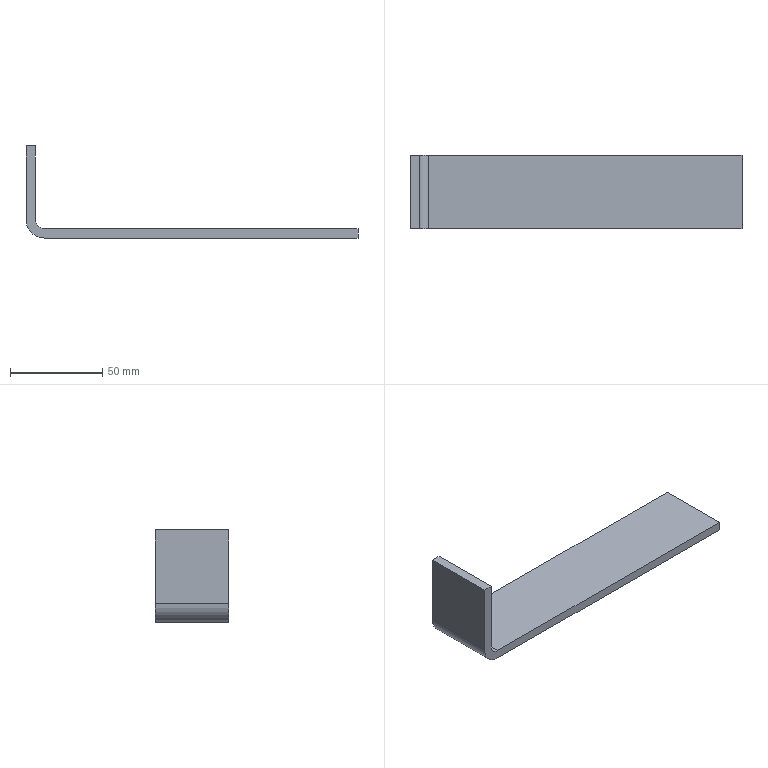Part | SolidWorks | features BaseBody 1 | 1 solid | 10 faces | box 180 x 40 x 50 mm | volume 44356 mm3 | plane 8 | cylinder 2 | commonest cylinder face diameters 10 x1 20 x1
STEP:
#1=CARTESIAN_POINT('',(0.,40.,0.));
#2=VERTEX_POINT('',#1);
#3=CARTESIAN_POINT('',(-170.,40.,0.));
#4=VERTEX_POINT('',#3);
#5=CARTESIAN_POINT('',(-90.,40.,0.));
#6=DIRECTION('',(-1.,0.,0.));
#7=VECTOR('',#6,1000.);
#8=LINE('',#5,#7);
#9=EDGE_CURVE('',#2,#4,#8,.T.);
#10=ORIENTED_EDGE('',*,*,#9,.F.);
#11=CARTESIAN_POINT('',(0.,0.,0.));
#12=VERTEX_POINT('',#11);
#13=CARTESIAN_POINT('',(0.,20.,0.));
#14=DIRECTION('',(0.,1.,0.));
#15=VECTOR('',#14,1000.);
#16=LINE('',#13,#15);
#17=EDGE_CURVE('',#12,#2,#16,.T.);
#18=ORIENTED_EDGE('',*,*,#17,.F.);
#19=CARTESIAN_POINT('',(-170.,0.,0.));
#20=VERTEX_POINT('',#19);
#21=CARTESIAN_POINT('',(-90.,0.,0.));
#22=DIRECTION('',(1.,0.,0.));
#23=VECTOR('',#22,1000.);
#24=LINE('',#21,#23);
#25=EDGE_CURVE('',#20,#12,#24,.T.);
#26=ORIENTED_EDGE('',*,*,#25,.F.);
#27=CARTESIAN_POINT('',(-170.,20.,0.));
#28=DIRECTION('',(0.,-1.,0.));
#29=VECTOR('',#28,1000.);
#30=LINE('',#27,#29);
#31=EDGE_CURVE('',#4,#20,#30,.T.);
#32=ORIENTED_EDGE('',*,*,#31,.F.);
#33=EDGE_LOOP('',(#10,#18,#26,#32));
#34=FACE_OUTER_BOUND('',#33,.T.);
#35=CARTESIAN_POINT('',(-90.,20.,0.));
#36=DIRECTION('',(0.,0.,1.));
#37=DIRECTION('',(1.,0.,0.));
#38=AXIS2_PLACEMENT_3D('',#35,#36,#37);
#39=PLANE('',#38);
#40=ADVANCED_FACE('',(#34),#39,.F.);
#41=ORIENTED_EDGE('',*,*,#31,.T.);
#42=CARTESIAN_POINT('',(-180.,0.,10.));
#43=VERTEX_POINT('',#42);
#44=CARTESIAN_POINT('',(-170.,0.,10.));
#45=DIRECTION('',(0.,1.,0.));
#46=DIRECTION('',(0.,0.,1.));
#47=AXIS2_PLACEMENT_3D('',#44,#45,#46);
#48=CIRCLE('',#47,10.);
#49=EDGE_CURVE('',#20,#43,#48,.T.);
#50=ORIENTED_EDGE('',*,*,#49,.T.);
#51=CARTESIAN_POINT('',(-180.,40.,10.));
#52=VERTEX_POINT('',#51);
#53=CARTESIAN_POINT('',(-180.,20.,10.));
#54=DIRECTION('',(0.,1.,0.));
#55=VECTOR('',#54,1000.);
#56=LINE('',#53,#55);
#57=EDGE_CURVE('',#43,#52,#56,.T.);
#58=ORIENTED_EDGE('',*,*,#57,.T.);
#59=CARTESIAN_POINT('',(-170.,40.,10.));
#60=DIRECTION('',(0.,-1.,0.));
#61=DIRECTION('',(0.,0.,1.));
#62=AXIS2_PLACEMENT_3D('',#59,#60,#61);
#63=CIRCLE('',#62,10.);
#64=EDGE_CURVE('',#52,#4,#63,.T.);
#65=ORIENTED_EDGE('',*,*,#64,.T.);
#66=EDGE_LOOP('',(#41,#50,#58,#65));
#67=FACE_OUTER_BOUND('',#66,.T.);
#68=CARTESIAN_POINT('',(-170.,20.,10.));
#69=DIRECTION('',(0.,1.,0.));
#70=DIRECTION('',(0.,0.,1.));
#71=AXIS2_PLACEMENT_3D('',#68,#69,#70);
#72=CYLINDRICAL_SURFACE('',#71,10.);
#73=ADVANCED_FACE('',(#67),#72,.T.);
#74=CARTESIAN_POINT('',(0.,40.,5.));
#75=VERTEX_POINT('',#74);
#76=CARTESIAN_POINT('',(0.,40.,0.));
#77=DIRECTION('',(0.,0.,-1.));
#78=VECTOR('',#77,1000.);
#79=LINE('',#76,#78);
#80=EDGE_CURVE('',#75,#2,#79,.T.);
#81=ORIENTED_EDGE('',*,*,#80,.T.);
#82=ORIENTED_EDGE('',*,*,#9,.T.);
#83=ORIENTED_EDGE('',*,*,#64,.F.);
#84=CARTESIAN_POINT('',(-180.,40.,50.));
#85=VERTEX_POINT('',#84);
#86=CARTESIAN_POINT('',(-180.,40.,24.345));
#87=DIRECTION('',(0.,0.,1.));
#88=VECTOR('',#87,1000.);
#89=LINE('',#86,#88);
#90=EDGE_CURVE('',#52,#85,#89,.T.);
#91=ORIENTED_EDGE('',*,*,#90,.T.);
#92=CARTESIAN_POINT('',(-175.,40.,50.));
#93=VERTEX_POINT('',#92);
#94=CARTESIAN_POINT('',(-175.,40.,50.));
#95=DIRECTION('',(1.,0.,0.));
#96=VECTOR('',#95,1000.);
#97=LINE('',#94,#96);
#98=EDGE_CURVE('',#85,#93,#97,.T.);
#99=ORIENTED_EDGE('',*,*,#98,.T.);
#100=CARTESIAN_POINT('',(-175.,40.,10.));
#101=VERTEX_POINT('',#100);
#102=CARTESIAN_POINT('',(-175.,40.,10.));
#103=DIRECTION('',(0.,0.,-1.));
#104=VECTOR('',#103,1000.);
#105=LINE('',#102,#104);
#106=EDGE_CURVE('',#93,#101,#105,.T.);
#107=ORIENTED_EDGE('',*,*,#106,.T.);
#108=CARTESIAN_POINT('',(-170.,40.,5.));
#109=VERTEX_POINT('',#108);
#110=CARTESIAN_POINT('',(-170.,40.,10.));
#111=DIRECTION('',(0.,-1.,0.));
#112=DIRECTION('',(0.,0.,1.));
#113=AXIS2_PLACEMENT_3D('',#110,#111,#112);
#114=CIRCLE('',#113,5.);
#115=EDGE_CURVE('',#101,#109,#114,.T.);
#116=ORIENTED_EDGE('',*,*,#115,.T.);
#117=CARTESIAN_POINT('',(-180.,40.,5.));
#118=DIRECTION('',(1.,0.,0.));
#119=VECTOR('',#118,1000.);
#120=LINE('',#117,#119);
#121=EDGE_CURVE('',#109,#75,#120,.T.);
#122=ORIENTED_EDGE('',*,*,#121,.T.);
#123=EDGE_LOOP('',(#81,#82,#83,#91,#99,#107,#116,#122));
#124=FACE_OUTER_BOUND('',#123,.T.);
#125=CARTESIAN_POINT('',(-180.,40.,0.));
#126=DIRECTION('',(0.,1.,0.));
#127=DIRECTION('',(-1.,0.,0.));
#128=AXIS2_PLACEMENT_3D('',#125,#126,#127);
#129=PLANE('',#128);
#130=ADVANCED_FACE('',(#124),#129,.T.);
#131=ORIENTED_EDGE('',*,*,#17,.T.);
#132=ORIENTED_EDGE('',*,*,#80,.F.);
#133=CARTESIAN_POINT('',(0.,0.,5.));
#134=VERTEX_POINT('',#133);
#135=CARTESIAN_POINT('',(0.,40.,5.));
#136=DIRECTION('',(0.,-1.,0.));
#137=VECTOR('',#136,1000.);
#138=LINE('',#135,#137);
#139=EDGE_CURVE('',#75,#134,#138,.T.);
#140=ORIENTED_EDGE('',*,*,#139,.T.);
#141=CARTESIAN_POINT('',(0.,0.,0.));
#142=DIRECTION('',(0.,0.,-1.));
#143=VECTOR('',#142,1000.);
#144=LINE('',#141,#143);
#145=EDGE_CURVE('',#134,#12,#144,.T.);
#146=ORIENTED_EDGE('',*,*,#145,.T.);
#147=EDGE_LOOP('',(#131,#132,#140,#146));
#148=FACE_OUTER_BOUND('',#147,.T.);
#149=CARTESIAN_POINT('',(0.,40.,0.));
#150=DIRECTION('',(1.,0.,0.));
#151=DIRECTION('',(0.,1.,0.));
#152=AXIS2_PLACEMENT_3D('',#149,#150,#151);
#153=PLANE('',#152);
#154=ADVANCED_FACE('',(#148),#153,.T.);
#155=ORIENTED_EDGE('',*,*,#145,.F.);
#156=CARTESIAN_POINT('',(-170.,0.,5.));
#157=VERTEX_POINT('',#156);
#158=CARTESIAN_POINT('',(0.,0.,5.));
#159=DIRECTION('',(-1.,0.,0.));
#160=VECTOR('',#159,1000.);
#161=LINE('',#158,#160);
#162=EDGE_CURVE('',#134,#157,#161,.T.);
#163=ORIENTED_EDGE('',*,*,#162,.T.);
#164=CARTESIAN_POINT('',(-175.,0.,10.));
#165=VERTEX_POINT('',#164);
#166=CARTESIAN_POINT('',(-170.,0.,10.));
#167=DIRECTION('',(0.,1.,0.));
#168=DIRECTION('',(0.,0.,1.));
#169=AXIS2_PLACEMENT_3D('',#166,#167,#168);
#170=CIRCLE('',#169,5.);
#171=EDGE_CURVE('',#157,#165,#170,.T.);
#172=ORIENTED_EDGE('',*,*,#171,.T.);
#173=CARTESIAN_POINT('',(-175.,0.,50.));
#174=VERTEX_POINT('',#173);
#175=CARTESIAN_POINT('',(-175.,0.,10.));
#176=DIRECTION('',(0.,0.,1.));
#177=VECTOR('',#176,1000.);
#178=LINE('',#175,#177);
#179=EDGE_CURVE('',#165,#174,#178,.T.);
#180=ORIENTED_EDGE('',*,*,#179,.T.);
#181=CARTESIAN_POINT('',(-180.,0.,50.));
#182=VERTEX_POINT('',#181);
#183=CARTESIAN_POINT('',(-175.,0.,50.));
#184=DIRECTION('',(-1.,0.,0.));
#185=VECTOR('',#184,1000.);
#186=LINE('',#183,#185);
#187=EDGE_CURVE('',#174,#182,#186,.T.);
#188=ORIENTED_EDGE('',*,*,#187,.T.);
#189=CARTESIAN_POINT('',(-180.,0.,24.345));
#190=DIRECTION('',(0.,0.,-1.));
#191=VECTOR('',#190,1000.);
#192=LINE('',#189,#191);
#193=EDGE_CURVE('',#182,#43,#192,.T.);
#194=ORIENTED_EDGE('',*,*,#193,.T.);
#195=ORIENTED_EDGE('',*,*,#49,.F.);
#196=ORIENTED_EDGE('',*,*,#25,.T.);
#197=EDGE_LOOP('',(#155,#163,#172,#180,#188,#194,#195,#196));
#198=FACE_OUTER_BOUND('',#197,.T.);
#199=CARTESIAN_POINT('',(0.,0.,0.));
#200=DIRECTION('',(0.,-1.,0.));
#201=DIRECTION('',(1.,0.,0.));
#202=AXIS2_PLACEMENT_3D('',#199,#200,#201);
#203=PLANE('',#202);
#204=ADVANCED_FACE('',(#198),#203,.T.);
#205=ORIENTED_EDGE('',*,*,#193,.F.);
#206=CARTESIAN_POINT('',(-180.,20.,50.));
#207=DIRECTION('',(0.,-1.,0.));
#208=VECTOR('',#207,1000.);
#209=LINE('',#206,#208);
#210=EDGE_CURVE('',#85,#182,#209,.T.);
#211=ORIENTED_EDGE('',*,*,#210,.F.);
#212=ORIENTED_EDGE('',*,*,#90,.F.);
#213=ORIENTED_EDGE('',*,*,#57,.F.);
#214=EDGE_LOOP('',(#205,#211,#212,#213));
#215=FACE_OUTER_BOUND('',#214,.T.);
#216=CARTESIAN_POINT('',(-180.,20.,24.345));
#217=DIRECTION('',(1.,0.,0.));
#218=DIRECTION('',(0.,0.,-1.));
#219=AXIS2_PLACEMENT_3D('',#216,#217,#218);
#220=PLANE('',#219);
#221=ADVANCED_FACE('',(#215),#220,.F.);
#222=ORIENTED_EDGE('',*,*,#139,.F.);
#223=ORIENTED_EDGE('',*,*,#121,.F.);
#224=CARTESIAN_POINT('',(-170.,20.,5.));
#225=DIRECTION('',(0.,-1.,0.));
#226=VECTOR('',#225,1000.);
#227=LINE('',#224,#226);
#228=EDGE_CURVE('',#109,#157,#227,.T.);
#229=ORIENTED_EDGE('',*,*,#228,.T.);
#230=ORIENTED_EDGE('',*,*,#162,.F.);
#231=EDGE_LOOP('',(#222,#223,#229,#230));
#232=FACE_OUTER_BOUND('',#231,.T.);
#233=CARTESIAN_POINT('',(-90.,20.,5.));
#234=DIRECTION('',(0.,0.,1.));
#235=DIRECTION('',(1.,0.,0.));
#236=AXIS2_PLACEMENT_3D('',#233,#234,#235);
#237=PLANE('',#236);
#238=ADVANCED_FACE('',(#232),#237,.T.);
#239=ORIENTED_EDGE('',*,*,#171,.F.);
#240=ORIENTED_EDGE('',*,*,#228,.F.);
#241=ORIENTED_EDGE('',*,*,#115,.F.);
#242=CARTESIAN_POINT('',(-175.,20.,10.));
#243=DIRECTION('',(0.,1.,0.));
#244=VECTOR('',#243,1000.);
#245=LINE('',#242,#244);
#246=EDGE_CURVE('',#165,#101,#245,.T.);
#247=ORIENTED_EDGE('',*,*,#246,.F.);
#248=EDGE_LOOP('',(#239,#240,#241,#247));
#249=FACE_OUTER_BOUND('',#248,.T.);
#250=CARTESIAN_POINT('',(-170.,20.,10.));
#251=DIRECTION('',(0.,1.,0.));
#252=DIRECTION('',(0.,0.,1.));
#253=AXIS2_PLACEMENT_3D('',#250,#251,#252);
#254=CYLINDRICAL_SURFACE('',#253,5.);
#255=ADVANCED_FACE('',(#249),#254,.F.);
#256=CARTESIAN_POINT('',(-175.,40.,50.));
#257=DIRECTION('',(0.,1.,0.));
#258=VECTOR('',#257,1000.);
#259=LINE('',#256,#258);
#260=EDGE_CURVE('',#174,#93,#259,.T.);
#261=ORIENTED_EDGE('',*,*,#260,.T.);
#262=ORIENTED_EDGE('',*,*,#98,.F.);
#263=ORIENTED_EDGE('',*,*,#210,.T.);
#264=ORIENTED_EDGE('',*,*,#187,.F.);
#265=EDGE_LOOP('',(#261,#262,#263,#264));
#266=FACE_OUTER_BOUND('',#265,.T.);
#267=CARTESIAN_POINT('',(-175.,40.,50.));
#268=DIRECTION('',(0.,0.,1.));
#269=DIRECTION('',(1.,0.,0.));
#270=AXIS2_PLACEMENT_3D('',#267,#268,#269);
#271=PLANE('',#270);
#272=ADVANCED_FACE('',(#266),#271,.T.);
#273=ORIENTED_EDGE('',*,*,#260,.F.);
#274=ORIENTED_EDGE('',*,*,#179,.F.);
#275=ORIENTED_EDGE('',*,*,#246,.T.);
#276=ORIENTED_EDGE('',*,*,#106,.F.);
#277=EDGE_LOOP('',(#273,#274,#275,#276));
#278=FACE_OUTER_BOUND('',#277,.T.);
#279=CARTESIAN_POINT('',(-175.,20.,24.345));
#280=DIRECTION('',(1.,0.,0.));
#281=DIRECTION('',(0.,0.,-1.));
#282=AXIS2_PLACEMENT_3D('',#279,#280,#281);
#283=PLANE('',#282);
#284=ADVANCED_FACE('',(#278),#283,.T.);
#285=CLOSED_SHELL('',(#40,#73,#130,#154,#204,#221,#238,#255,#272,#284));
#286=MANIFOLD_SOLID_BREP('',#285);
#287=CARTESIAN_POINT('',(0.,0.,0.));
#288=DIRECTION('',(0.,0.,1.));
#289=DIRECTION('',(1.,0.,0.));
#290=AXIS2_PLACEMENT_3D('',#287,#288,#289);
#291=(LENGTH_UNIT()NAMED_UNIT(*)SI_UNIT(.MILLI.,.METRE.));
#292=UNCERTAINTY_MEASURE_WITH_UNIT(LENGTH_MEASURE(0.00001),#291,'','');
#293=(NAMED_UNIT(*)PLANE_ANGLE_UNIT()SI_UNIT($,.RADIAN.));
#294=(NAMED_UNIT(*)SI_UNIT($,.STERADIAN.)SOLID_ANGLE_UNIT());
#295=(GEOMETRIC_REPRESENTATION_CONTEXT(3)GLOBAL_UNCERTAINTY_ASSIGNED_CONTEXT((#292))GLOBAL_UNIT_ASSIGNED_CONTEXT((#291,#293,#294))REPRESENTATION_CONTEXT('',''));
#296=ADVANCED_BREP_SHAPE_REPRESENTATION('',(#286,#290),#295);